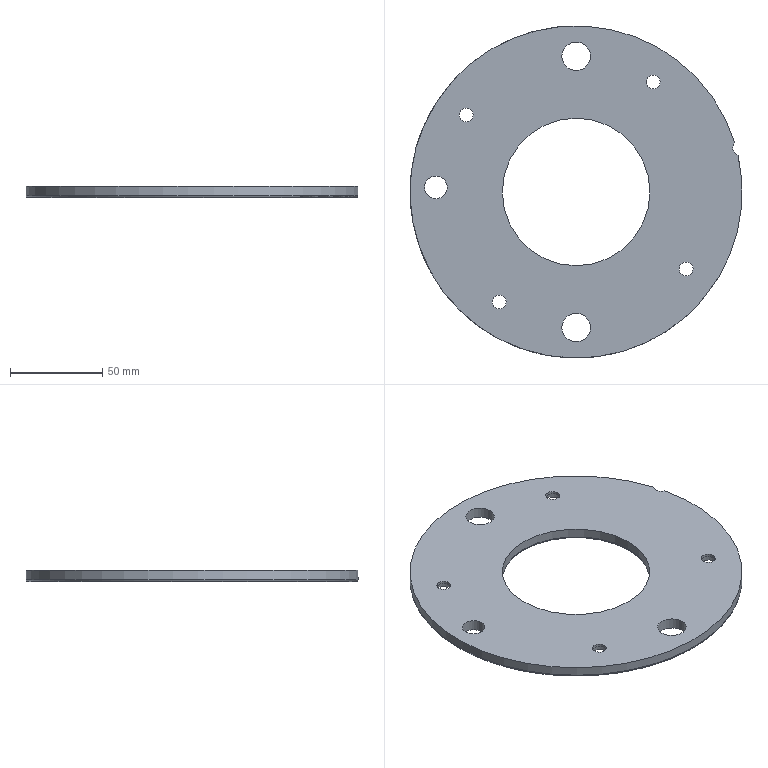Part | STEP file | Slide_plate | 1 solid | 23 faces | box 180 x 180 x 6 mm | volume 116281 mm3 | cylinder 14 | plane 6 | torus 3 | commonest cylinder face diameters 7.5 x4 14 x4 15.5 x2 8 x1 12.25 x1 80 x1